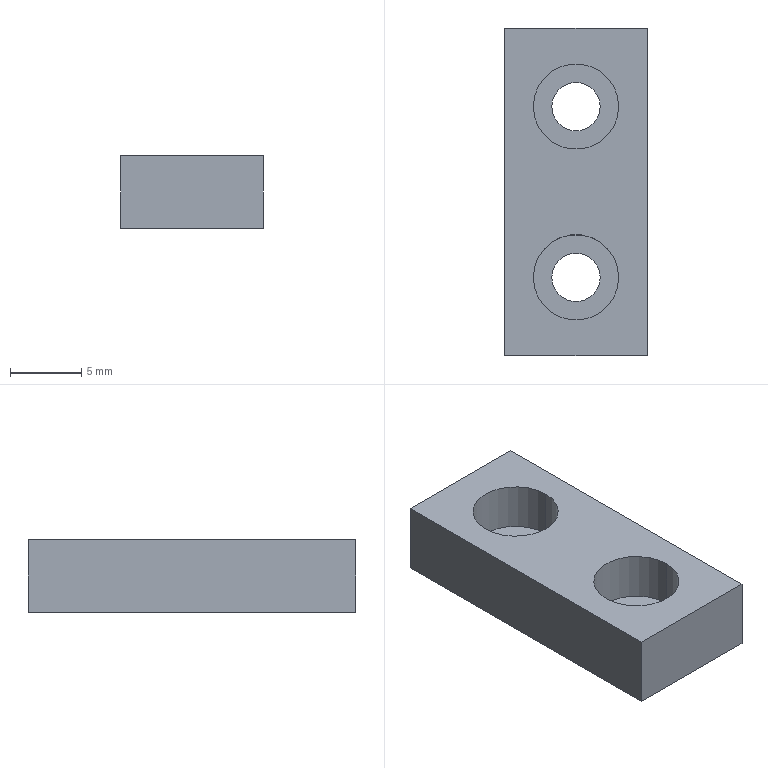Part | STEP file | 2041 Bag feed assist block | 1 solid | 16 faces | box 10 x 23 x 5.1 mm | volume 949.865 mm3 | cylinder 8 | plane 8 | commonest cylinder face diameters 3.4 x4 6 x4
STEP:
#1=CARTESIAN_POINT('',(0.,0.,0.));
#2=DIRECTION('',(0.,0.,1.));
#3=DIRECTION('',(1.,0.,0.));
#4=AXIS2_PLACEMENT_3D('',#1,#2,#3);
#5=CARTESIAN_POINT('',(3.,6.,1.7));
#6=VERTEX_POINT('',#5);
#7=CARTESIAN_POINT('',(3.,6.,5.1));
#8=VERTEX_POINT('',#7);
#9=CARTESIAN_POINT('',(3.,6.,5.1));
#10=DIRECTION('',(0.,0.,1.));
#11=VECTOR('',#10,1.);
#12=LINE('',#9,#11);
#13=CARTESIAN_POINT('',(0.,6.,5.1));
#14=DIRECTION('',(0.,0.,1.));
#15=DIRECTION('',(1.,0.,0.));
#16=AXIS2_PLACEMENT_3D('',#13,#14,#15);
#17=CYLINDRICAL_SURFACE('',#16,3.);
#18=CARTESIAN_POINT('',(6.283,0.));
#19=DIRECTION('',(0.,1.));
#20=VECTOR('',#19,1.);
#21=LINE('',#18,#20);
#22=(GEOMETRIC_REPRESENTATION_CONTEXT(2)PARAMETRIC_REPRESENTATION_CONTEXT()REPRESENTATION_CONTEXT('',''));
#23=DEFINITIONAL_REPRESENTATION('',(#21),#22);
#24=PCURVE('',#17,#23);
#25=CARTESIAN_POINT('',(0.,6.,5.1));
#26=DIRECTION('',(0.,0.,1.));
#27=DIRECTION('',(1.,0.,0.));
#28=AXIS2_PLACEMENT_3D('',#25,#26,#27);
#29=CYLINDRICAL_SURFACE('',#28,3.);
#30=CARTESIAN_POINT('',(0.,0.));
#31=DIRECTION('',(0.,1.));
#32=VECTOR('',#31,1.);
#33=LINE('',#30,#32);
#34=(GEOMETRIC_REPRESENTATION_CONTEXT(2)PARAMETRIC_REPRESENTATION_CONTEXT()REPRESENTATION_CONTEXT('',''));
#35=DEFINITIONAL_REPRESENTATION('',(#33),#34);
#36=PCURVE('',#29,#35);
#37=SURFACE_CURVE('',#12,(#24,#36),.PCURVE_S1.);
#38=EDGE_CURVE('',#6,#8,#37,.T.);
#39=ORIENTED_EDGE('',*,*,#38,.T.);
#40=CARTESIAN_POINT('',(-3.,6.,5.1));
#41=VERTEX_POINT('',#40);
#42=CARTESIAN_POINT('',(0.,6.,5.1));
#43=DIRECTION('',(0.,0.,1.));
#44=DIRECTION('',(1.,0.,0.));
#45=AXIS2_PLACEMENT_3D('',#42,#43,#44);
#46=CIRCLE('',#45,3.);
#47=CARTESIAN_POINT('',(0.,0.));
#48=DIRECTION('',(1.,0.));
#49=VECTOR('',#48,1.);
#50=LINE('',#47,#49);
#51=(GEOMETRIC_REPRESENTATION_CONTEXT(2)PARAMETRIC_REPRESENTATION_CONTEXT()REPRESENTATION_CONTEXT('',''));
#52=DEFINITIONAL_REPRESENTATION('',(#50),#51);
#53=PCURVE('',#17,#52);
#54=CARTESIAN_POINT('',(0.,0.,5.1));
#55=DIRECTION('',(0.,0.,-1.));
#56=DIRECTION('',(-1.,0.,0.));
#57=AXIS2_PLACEMENT_3D('',#54,#55,#56);
#58=PLANE('',#57);
#59=CARTESIAN_POINT('',(-3.,6.));
#60=CARTESIAN_POINT('',(-3.,11.196));
#61=CARTESIAN_POINT('',(1.5,8.598));
#62=CARTESIAN_POINT('',(6.,6.));
#63=CARTESIAN_POINT('',(1.5,3.402));
#64=CARTESIAN_POINT('',(-3.,0.8038));
#65=CARTESIAN_POINT('',(-3.,6.));
#66=(BOUNDED_CURVE()B_SPLINE_CURVE(2,(#59,#60,#61,#62,#63,#64,#65),.UNSPECIFIED.,.T.,.F.)B_SPLINE_CURVE_WITH_KNOTS((1,2,2,2,2,1),(-2.094,0.,2.094,4.189,6.283,8.378),.UNSPECIFIED.)CURVE()GEOMETRIC_REPRESENTATION_ITEM()RATIONAL_B_SPLINE_CURVE((1.,0.5,1.,0.5,1.,0.5,1.))REPRESENTATION_ITEM(''));
#67=(GEOMETRIC_REPRESENTATION_CONTEXT(2)PARAMETRIC_REPRESENTATION_CONTEXT()REPRESENTATION_CONTEXT('',''));
#68=DEFINITIONAL_REPRESENTATION('',(#66),#67);
#69=PCURVE('',#58,#68);
#70=SURFACE_CURVE('',#46,(#53,#69),.PCURVE_S1.);
#71=EDGE_CURVE('',#41,#8,#70,.T.);
#72=ORIENTED_EDGE('',*,*,#71,.F.);
#73=CARTESIAN_POINT('',(-3.,6.,1.7));
#74=VERTEX_POINT('',#73);
#75=CARTESIAN_POINT('',(-3.,6.,5.1));
#76=DIRECTION('',(0.,0.,1.));
#77=VECTOR('',#76,1.);
#78=LINE('',#75,#77);
#79=CARTESIAN_POINT('',(3.142,0.));
#80=DIRECTION('',(0.,1.));
#81=VECTOR('',#80,1.);
#82=LINE('',#79,#81);
#83=(GEOMETRIC_REPRESENTATION_CONTEXT(2)PARAMETRIC_REPRESENTATION_CONTEXT()REPRESENTATION_CONTEXT('',''));
#84=DEFINITIONAL_REPRESENTATION('',(#82),#83);
#85=PCURVE('',#17,#84);
#86=CARTESIAN_POINT('',(3.142,0.));
#87=DIRECTION('',(0.,1.));
#88=VECTOR('',#87,1.);
#89=LINE('',#86,#88);
#90=(GEOMETRIC_REPRESENTATION_CONTEXT(2)PARAMETRIC_REPRESENTATION_CONTEXT()REPRESENTATION_CONTEXT('',''));
#91=DEFINITIONAL_REPRESENTATION('',(#89),#90);
#92=PCURVE('',#29,#91);
#93=SURFACE_CURVE('',#78,(#85,#92),.PCURVE_S1.);
#94=EDGE_CURVE('',#74,#41,#93,.T.);
#95=ORIENTED_EDGE('',*,*,#94,.F.);
#96=CARTESIAN_POINT('',(0.,6.,1.7));
#97=DIRECTION('',(0.,0.,1.));
#98=DIRECTION('',(1.,0.,0.));
#99=AXIS2_PLACEMENT_3D('',#96,#97,#98);
#100=CIRCLE('',#99,3.);
#101=CARTESIAN_POINT('',(0.,-3.4));
#102=DIRECTION('',(1.,0.));
#103=VECTOR('',#102,1.);
#104=LINE('',#101,#103);
#105=(GEOMETRIC_REPRESENTATION_CONTEXT(2)PARAMETRIC_REPRESENTATION_CONTEXT()REPRESENTATION_CONTEXT('',''));
#106=DEFINITIONAL_REPRESENTATION('',(#104),#105);
#107=PCURVE('',#17,#106);
#108=CARTESIAN_POINT('',(1.7,6.,1.7));
#109=DIRECTION('',(0.,0.,-1.));
#110=DIRECTION('',(-1.,0.,0.));
#111=AXIS2_PLACEMENT_3D('',#108,#109,#110);
#112=PLANE('',#111);
#113=CARTESIAN_POINT('',(-1.3,0.));
#114=CARTESIAN_POINT('',(-1.3,5.196));
#115=CARTESIAN_POINT('',(3.2,2.598));
#116=CARTESIAN_POINT('',(7.7,0.));
#117=CARTESIAN_POINT('',(3.2,-2.598));
#118=CARTESIAN_POINT('',(-1.3,-5.196));
#119=CARTESIAN_POINT('',(-1.3,0.));
#120=(BOUNDED_CURVE()B_SPLINE_CURVE(2,(#113,#114,#115,#116,#117,#118,#119),.UNSPECIFIED.,.T.,.F.)B_SPLINE_CURVE_WITH_KNOTS((1,2,2,2,2,1),(-2.094,0.,2.094,4.189,6.283,8.378),.UNSPECIFIED.)CURVE()GEOMETRIC_REPRESENTATION_ITEM()RATIONAL_B_SPLINE_CURVE((1.,0.5,1.,0.5,1.,0.5,1.))REPRESENTATION_ITEM(''));
#121=(GEOMETRIC_REPRESENTATION_CONTEXT(2)PARAMETRIC_REPRESENTATION_CONTEXT()REPRESENTATION_CONTEXT('',''));
#122=DEFINITIONAL_REPRESENTATION('',(#120),#121);
#123=PCURVE('',#112,#122);
#124=SURFACE_CURVE('',#100,(#107,#123),.PCURVE_S1.);
#125=EDGE_CURVE('',#74,#6,#124,.T.);
#126=ORIENTED_EDGE('',*,*,#125,.T.);
#127=EDGE_LOOP('',(#39,#72,#95,#126));
#128=FACE_BOUND('',#127,.F.);
#129=ADVANCED_FACE('',(#128),#17,.F.);
#130=CARTESIAN_POINT('',(1.7,6.,0.));
#131=VERTEX_POINT('',#130);
#132=CARTESIAN_POINT('',(1.7,6.,1.7));
#133=VERTEX_POINT('',#132);
#134=CARTESIAN_POINT('',(1.7,6.,5.1));
#135=DIRECTION('',(0.,0.,1.));
#136=VECTOR('',#135,1.);
#137=LINE('',#134,#136);
#138=CARTESIAN_POINT('',(0.,6.,5.1));
#139=DIRECTION('',(0.,0.,1.));
#140=DIRECTION('',(1.,0.,0.));
#141=AXIS2_PLACEMENT_3D('',#138,#139,#140);
#142=CYLINDRICAL_SURFACE('',#141,1.7);
#143=CARTESIAN_POINT('',(6.283,0.));
#144=DIRECTION('',(0.,1.));
#145=VECTOR('',#144,1.);
#146=LINE('',#143,#145);
#147=(GEOMETRIC_REPRESENTATION_CONTEXT(2)PARAMETRIC_REPRESENTATION_CONTEXT()REPRESENTATION_CONTEXT('',''));
#148=DEFINITIONAL_REPRESENTATION('',(#146),#147);
#149=PCURVE('',#142,#148);
#150=CARTESIAN_POINT('',(0.,6.,5.1));
#151=DIRECTION('',(0.,0.,1.));
#152=DIRECTION('',(1.,0.,0.));
#153=AXIS2_PLACEMENT_3D('',#150,#151,#152);
#154=CYLINDRICAL_SURFACE('',#153,1.7);
#155=CARTESIAN_POINT('',(0.,0.));
#156=DIRECTION('',(0.,1.));
#157=VECTOR('',#156,1.);
#158=LINE('',#155,#157);
#159=(GEOMETRIC_REPRESENTATION_CONTEXT(2)PARAMETRIC_REPRESENTATION_CONTEXT()REPRESENTATION_CONTEXT('',''));
#160=DEFINITIONAL_REPRESENTATION('',(#158),#159);
#161=PCURVE('',#154,#160);
#162=SURFACE_CURVE('',#137,(#149,#161),.PCURVE_S1.);
#163=EDGE_CURVE('',#131,#133,#162,.T.);
#164=ORIENTED_EDGE('',*,*,#163,.T.);
#165=CARTESIAN_POINT('',(-1.7,6.,1.7));
#166=VERTEX_POINT('',#165);
#167=CARTESIAN_POINT('',(0.,6.,1.7));
#168=DIRECTION('',(0.,0.,1.));
#169=DIRECTION('',(1.,0.,0.));
#170=AXIS2_PLACEMENT_3D('',#167,#168,#169);
#171=CIRCLE('',#170,1.7);
#172=CARTESIAN_POINT('',(0.,-3.4));
#173=DIRECTION('',(1.,0.));
#174=VECTOR('',#173,1.);
#175=LINE('',#172,#174);
#176=(GEOMETRIC_REPRESENTATION_CONTEXT(2)PARAMETRIC_REPRESENTATION_CONTEXT()REPRESENTATION_CONTEXT('',''));
#177=DEFINITIONAL_REPRESENTATION('',(#175),#176);
#178=PCURVE('',#142,#177);
#179=CARTESIAN_POINT('',(0.,0.));
#180=CARTESIAN_POINT('',(0.,2.944));
#181=CARTESIAN_POINT('',(2.55,1.472));
#182=CARTESIAN_POINT('',(5.1,0.));
#183=CARTESIAN_POINT('',(2.55,-1.472));
#184=CARTESIAN_POINT('',(0.,-2.944));
#185=CARTESIAN_POINT('',(0.,0.));
#186=(BOUNDED_CURVE()B_SPLINE_CURVE(2,(#179,#180,#181,#182,#183,#184,#185),.UNSPECIFIED.,.T.,.F.)B_SPLINE_CURVE_WITH_KNOTS((1,2,2,2,2,1),(-2.094,0.,2.094,4.189,6.283,8.378),.UNSPECIFIED.)CURVE()GEOMETRIC_REPRESENTATION_ITEM()RATIONAL_B_SPLINE_CURVE((1.,0.5,1.,0.5,1.,0.5,1.))REPRESENTATION_ITEM(''));
#187=(GEOMETRIC_REPRESENTATION_CONTEXT(2)PARAMETRIC_REPRESENTATION_CONTEXT()REPRESENTATION_CONTEXT('',''));
#188=DEFINITIONAL_REPRESENTATION('',(#186),#187);
#189=PCURVE('',#112,#188);
#190=SURFACE_CURVE('',#171,(#178,#189),.PCURVE_S1.);
#191=EDGE_CURVE('',#166,#133,#190,.T.);
#192=ORIENTED_EDGE('',*,*,#191,.F.);
#193=CARTESIAN_POINT('',(-1.7,6.,0.));
#194=VERTEX_POINT('',#193);
#195=CARTESIAN_POINT('',(-1.7,6.,5.1));
#196=DIRECTION('',(0.,0.,1.));
#197=VECTOR('',#196,1.);
#198=LINE('',#195,#197);
#199=CARTESIAN_POINT('',(3.142,0.));
#200=DIRECTION('',(0.,1.));
#201=VECTOR('',#200,1.);
#202=LINE('',#199,#201);
#203=(GEOMETRIC_REPRESENTATION_CONTEXT(2)PARAMETRIC_REPRESENTATION_CONTEXT()REPRESENTATION_CONTEXT('',''));
#204=DEFINITIONAL_REPRESENTATION('',(#202),#203);
#205=PCURVE('',#142,#204);
#206=CARTESIAN_POINT('',(3.142,0.));
#207=DIRECTION('',(0.,1.));
#208=VECTOR('',#207,1.);
#209=LINE('',#206,#208);
#210=(GEOMETRIC_REPRESENTATION_CONTEXT(2)PARAMETRIC_REPRESENTATION_CONTEXT()REPRESENTATION_CONTEXT('',''));
#211=DEFINITIONAL_REPRESENTATION('',(#209),#210);
#212=PCURVE('',#154,#211);
#213=SURFACE_CURVE('',#198,(#205,#212),.PCURVE_S1.);
#214=EDGE_CURVE('',#194,#166,#213,.T.);
#215=ORIENTED_EDGE('',*,*,#214,.F.);
#216=CARTESIAN_POINT('',(0.,6.,0.));
#217=DIRECTION('',(0.,0.,1.));
#218=DIRECTION('',(1.,0.,0.));
#219=AXIS2_PLACEMENT_3D('',#216,#217,#218);
#220=CIRCLE('',#219,1.7);
#221=CARTESIAN_POINT('',(0.,-5.1));
#222=DIRECTION('',(1.,0.));
#223=VECTOR('',#222,1.);
#224=LINE('',#221,#223);
#225=(GEOMETRIC_REPRESENTATION_CONTEXT(2)PARAMETRIC_REPRESENTATION_CONTEXT()REPRESENTATION_CONTEXT('',''));
#226=DEFINITIONAL_REPRESENTATION('',(#224),#225);
#227=PCURVE('',#142,#226);
#228=CARTESIAN_POINT('',(0.,0.,0.));
#229=DIRECTION('',(0.,0.,-1.));
#230=DIRECTION('',(-1.,0.,0.));
#231=AXIS2_PLACEMENT_3D('',#228,#229,#230);
#232=PLANE('',#231);
#233=CARTESIAN_POINT('',(-1.7,6.));
#234=CARTESIAN_POINT('',(-1.7,8.944));
#235=CARTESIAN_POINT('',(0.85,7.472));
#236=CARTESIAN_POINT('',(3.4,6.));
#237=CARTESIAN_POINT('',(0.85,4.528));
#238=CARTESIAN_POINT('',(-1.7,3.056));
#239=CARTESIAN_POINT('',(-1.7,6.));
#240=(BOUNDED_CURVE()B_SPLINE_CURVE(2,(#233,#234,#235,#236,#237,#238,#239),.UNSPECIFIED.,.T.,.F.)B_SPLINE_CURVE_WITH_KNOTS((1,2,2,2,2,1),(-2.094,0.,2.094,4.189,6.283,8.378),.UNSPECIFIED.)CURVE()GEOMETRIC_REPRESENTATION_ITEM()RATIONAL_B_SPLINE_CURVE((1.,0.5,1.,0.5,1.,0.5,1.))REPRESENTATION_ITEM(''));
#241=(GEOMETRIC_REPRESENTATION_CONTEXT(2)PARAMETRIC_REPRESENTATION_CONTEXT()REPRESENTATION_CONTEXT('',''));
#242=DEFINITIONAL_REPRESENTATION('',(#240),#241);
#243=PCURVE('',#232,#242);
#244=SURFACE_CURVE('',#220,(#227,#243),.PCURVE_S1.);
#245=EDGE_CURVE('',#194,#131,#244,.T.);
#246=ORIENTED_EDGE('',*,*,#245,.T.);
#247=EDGE_LOOP('',(#164,#192,#215,#246));
#248=FACE_BOUND('',#247,.F.);
#249=ADVANCED_FACE('',(#248),#142,.F.);
#250=CARTESIAN_POINT('',(3.,-6.,1.7));
#251=VERTEX_POINT('',#250);
#252=CARTESIAN_POINT('',(3.,-6.,5.1));
#253=VERTEX_POINT('',#252);
#254=CARTESIAN_POINT('',(3.,-6.,5.1));
#255=DIRECTION('',(0.,0.,1.));
#256=VECTOR('',#255,1.);
#257=LINE('',#254,#256);
#258=CARTESIAN_POINT('',(0.,-6.,5.1));
#259=DIRECTION('',(0.,0.,1.));
#260=DIRECTION('',(1.,0.,0.));
#261=AXIS2_PLACEMENT_3D('',#258,#259,#260);
#262=CYLINDRICAL_SURFACE('',#261,3.);
#263=CARTESIAN_POINT('',(6.283,0.));
#264=DIRECTION('',(0.,1.));
#265=VECTOR('',#264,1.);
#266=LINE('',#263,#265);
#267=(GEOMETRIC_REPRESENTATION_CONTEXT(2)PARAMETRIC_REPRESENTATION_CONTEXT()REPRESENTATION_CONTEXT('',''));
#268=DEFINITIONAL_REPRESENTATION('',(#266),#267);
#269=PCURVE('',#262,#268);
#270=CARTESIAN_POINT('',(0.,-6.,5.1));
#271=DIRECTION('',(0.,0.,1.));
#272=DIRECTION('',(1.,0.,0.));
#273=AXIS2_PLACEMENT_3D('',#270,#271,#272);
#274=CYLINDRICAL_SURFACE('',#273,3.);
#275=CARTESIAN_POINT('',(0.,0.));
#276=DIRECTION('',(0.,1.));
#277=VECTOR('',#276,1.);
#278=LINE('',#275,#277);
#279=(GEOMETRIC_REPRESENTATION_CONTEXT(2)PARAMETRIC_REPRESENTATION_CONTEXT()REPRESENTATION_CONTEXT('',''));
#280=DEFINITIONAL_REPRESENTATION('',(#278),#279);
#281=PCURVE('',#274,#280);
#282=SURFACE_CURVE('',#257,(#269,#281),.PCURVE_S1.);
#283=EDGE_CURVE('',#251,#253,#282,.T.);
#284=ORIENTED_EDGE('',*,*,#283,.T.);
#285=CARTESIAN_POINT('',(-3.,-6.,5.1));
#286=VERTEX_POINT('',#285);
#287=CARTESIAN_POINT('',(0.,-6.,5.1));
#288=DIRECTION('',(0.,0.,1.));
#289=DIRECTION('',(1.,0.,0.));
#290=AXIS2_PLACEMENT_3D('',#287,#288,#289);
#291=CIRCLE('',#290,3.);
#292=CARTESIAN_POINT('',(0.,0.));
#293=DIRECTION('',(1.,0.));
#294=VECTOR('',#293,1.);
#295=LINE('',#292,#294);
#296=(GEOMETRIC_REPRESENTATION_CONTEXT(2)PARAMETRIC_REPRESENTATION_CONTEXT()REPRESENTATION_CONTEXT('',''));
#297=DEFINITIONAL_REPRESENTATION('',(#295),#296);
#298=PCURVE('',#262,#297);
#299=CARTESIAN_POINT('',(-3.,-6.));
#300=CARTESIAN_POINT('',(-3.,-0.8038));
#301=CARTESIAN_POINT('',(1.5,-3.402));
#302=CARTESIAN_POINT('',(6.,-6.));
#303=CARTESIAN_POINT('',(1.5,-8.598));
#304=CARTESIAN_POINT('',(-3.,-11.196));
#305=CARTESIAN_POINT('',(-3.,-6.));
#306=(BOUNDED_CURVE()B_SPLINE_CURVE(2,(#299,#300,#301,#302,#303,#304,#305),.UNSPECIFIED.,.T.,.F.)B_SPLINE_CURVE_WITH_KNOTS((1,2,2,2,2,1),(-2.094,0.,2.094,4.189,6.283,8.378),.UNSPECIFIED.)CURVE()GEOMETRIC_REPRESENTATION_ITEM()RATIONAL_B_SPLINE_CURVE((1.,0.5,1.,0.5,1.,0.5,1.))REPRESENTATION_ITEM(''));
#307=(GEOMETRIC_REPRESENTATION_CONTEXT(2)PARAMETRIC_REPRESENTATION_CONTEXT()REPRESENTATION_CONTEXT('',''));
#308=DEFINITIONAL_REPRESENTATION('',(#306),#307);
#309=PCURVE('',#58,#308);
#310=SURFACE_CURVE('',#291,(#298,#309),.PCURVE_S1.);
#311=EDGE_CURVE('',#286,#253,#310,.T.);
#312=ORIENTED_EDGE('',*,*,#311,.F.);
#313=CARTESIAN_POINT('',(-3.,-6.,1.7));
#314=VERTEX_POINT('',#313);
#315=CARTESIAN_POINT('',(-3.,-6.,5.1));
#316=DIRECTION('',(0.,0.,1.));
#317=VECTOR('',#316,1.);
#318=LINE('',#315,#317);
#319=CARTESIAN_POINT('',(3.142,0.));
#320=DIRECTION('',(0.,1.));
#321=VECTOR('',#320,1.);
#322=LINE('',#319,#321);
#323=(GEOMETRIC_REPRESENTATION_CONTEXT(2)PARAMETRIC_REPRESENTATION_CONTEXT()REPRESENTATION_CONTEXT('',''));
#324=DEFINITIONAL_REPRESENTATION('',(#322),#323);
#325=PCURVE('',#262,#324);
#326=CARTESIAN_POINT('',(3.142,0.));
#327=DIRECTION('',(0.,1.));
#328=VECTOR('',#327,1.);
#329=LINE('',#326,#328);
#330=(GEOMETRIC_REPRESENTATION_CONTEXT(2)PARAMETRIC_REPRESENTATION_CONTEXT()REPRESENTATION_CONTEXT('',''));
#331=DEFINITIONAL_REPRESENTATION('',(#329),#330);
#332=PCURVE('',#274,#331);
#333=SURFACE_CURVE('',#318,(#325,#332),.PCURVE_S1.);
#334=EDGE_CURVE('',#314,#286,#333,.T.);
#335=ORIENTED_EDGE('',*,*,#334,.F.);
#336=CARTESIAN_POINT('',(0.,-6.,1.7));
#337=DIRECTION('',(0.,0.,1.));
#338=DIRECTION('',(1.,0.,0.));
#339=AXIS2_PLACEMENT_3D('',#336,#337,#338);
#340=CIRCLE('',#339,3.);
#341=CARTESIAN_POINT('',(0.,-3.4));
#342=DIRECTION('',(1.,0.));
#343=VECTOR('',#342,1.);
#344=LINE('',#341,#343);
#345=(GEOMETRIC_REPRESENTATION_CONTEXT(2)PARAMETRIC_REPRESENTATION_CONTEXT()REPRESENTATION_CONTEXT('',''));
#346=DEFINITIONAL_REPRESENTATION('',(#344),#345);
#347=PCURVE('',#262,#346);
#348=CARTESIAN_POINT('',(1.7,-6.,1.7));
#349=DIRECTION('',(0.,0.,-1.));
#350=DIRECTION('',(-1.,0.,0.));
#351=AXIS2_PLACEMENT_3D('',#348,#349,#350);
#352=PLANE('',#351);
#353=CARTESIAN_POINT('',(-1.3,0.));
#354=CARTESIAN_POINT('',(-1.3,5.196));
#355=CARTESIAN_POINT('',(3.2,2.598));
#356=CARTESIAN_POINT('',(7.7,0.));
#357=CARTESIAN_POINT('',(3.2,-2.598));
#358=CARTESIAN_POINT('',(-1.3,-5.196));
#359=CARTESIAN_POINT('',(-1.3,0.));
#360=(BOUNDED_CURVE()B_SPLINE_CURVE(2,(#353,#354,#355,#356,#357,#358,#359),.UNSPECIFIED.,.T.,.F.)B_SPLINE_CURVE_WITH_KNOTS((1,2,2,2,2,1),(-2.094,0.,2.094,4.189,6.283,8.378),.UNSPECIFIED.)CURVE()GEOMETRIC_REPRESENTATION_ITEM()RATIONAL_B_SPLINE_CURVE((1.,0.5,1.,0.5,1.,0.5,1.))REPRESENTATION_ITEM(''));
#361=(GEOMETRIC_REPRESENTATION_CONTEXT(2)PARAMETRIC_REPRESENTATION_CONTEXT()REPRESENTATION_CONTEXT('',''));
#362=DEFINITIONAL_REPRESENTATION('',(#360),#361);
#363=PCURVE('',#352,#362);
#364=SURFACE_CURVE('',#340,(#347,#363),.PCURVE_S1.);
#365=EDGE_CURVE('',#314,#251,#364,.T.);
#366=ORIENTED_EDGE('',*,*,#365,.T.);
#367=EDGE_LOOP('',(#284,#312,#335,#366));
#368=FACE_BOUND('',#367,.F.);
#369=ADVANCED_FACE('',(#368),#262,.F.);
#370=CARTESIAN_POINT('',(1.7,-6.,0.));
#371=VERTEX_POINT('',#370);
#372=CARTESIAN_POINT('',(1.7,-6.,1.7));
#373=VERTEX_POINT('',#372);
#374=CARTESIAN_POINT('',(1.7,-6.,5.1));
#375=DIRECTION('',(0.,0.,1.));
#376=VECTOR('',#375,1.);
#377=LINE('',#374,#376);
#378=CARTESIAN_POINT('',(0.,-6.,5.1));
#379=DIRECTION('',(0.,0.,1.));
#380=DIRECTION('',(1.,0.,0.));
#381=AXIS2_PLACEMENT_3D('',#378,#379,#380);
#382=CYLINDRICAL_SURFACE('',#381,1.7);
#383=CARTESIAN_POINT('',(6.283,0.));
#384=DIRECTION('',(0.,1.));
#385=VECTOR('',#384,1.);
#386=LINE('',#383,#385);
#387=(GEOMETRIC_REPRESENTATION_CONTEXT(2)PARAMETRIC_REPRESENTATION_CONTEXT()REPRESENTATION_CONTEXT('',''));
#388=DEFINITIONAL_REPRESENTATION('',(#386),#387);
#389=PCURVE('',#382,#388);
#390=CARTESIAN_POINT('',(0.,-6.,5.1));
#391=DIRECTION('',(0.,0.,1.));
#392=DIRECTION('',(1.,0.,0.));
#393=AXIS2_PLACEMENT_3D('',#390,#391,#392);
#394=CYLINDRICAL_SURFACE('',#393,1.7);
#395=CARTESIAN_POINT('',(0.,0.));
#396=DIRECTION('',(0.,1.));
#397=VECTOR('',#396,1.);
#398=LINE('',#395,#397);
#399=(GEOMETRIC_REPRESENTATION_CONTEXT(2)PARAMETRIC_REPRESENTATION_CONTEXT()REPRESENTATION_CONTEXT('',''));
#400=DEFINITIONAL_REPRESENTATION('',(#398),#399);
#401=PCURVE('',#394,#400);
#402=SURFACE_CURVE('',#377,(#389,#401),.PCURVE_S1.);
#403=EDGE_CURVE('',#371,#373,#402,.T.);
#404=ORIENTED_EDGE('',*,*,#403,.T.);
#405=CARTESIAN_POINT('',(-1.7,-6.,1.7));
#406=VERTEX_POINT('',#405);
#407=CARTESIAN_POINT('',(0.,-6.,1.7));
#408=DIRECTION('',(0.,0.,1.));
#409=DIRECTION('',(1.,0.,0.));
#410=AXIS2_PLACEMENT_3D('',#407,#408,#409);
#411=CIRCLE('',#410,1.7);
#412=CARTESIAN_POINT('',(0.,-3.4));
#413=DIRECTION('',(1.,0.));
#414=VECTOR('',#413,1.);
#415=LINE('',#412,#414);
#416=(GEOMETRIC_REPRESENTATION_CONTEXT(2)PARAMETRIC_REPRESENTATION_CONTEXT()REPRESENTATION_CONTEXT('',''));
#417=DEFINITIONAL_REPRESENTATION('',(#415),#416);
#418=PCURVE('',#382,#417);
#419=CARTESIAN_POINT('',(0.,0.));
#420=CARTESIAN_POINT('',(0.,2.944));
#421=CARTESIAN_POINT('',(2.55,1.472));
#422=CARTESIAN_POINT('',(5.1,0.));
#423=CARTESIAN_POINT('',(2.55,-1.472));
#424=CARTESIAN_POINT('',(0.,-2.944));
#425=CARTESIAN_POINT('',(0.,0.));
#426=(BOUNDED_CURVE()B_SPLINE_CURVE(2,(#419,#420,#421,#422,#423,#424,#425),.UNSPECIFIED.,.T.,.F.)B_SPLINE_CURVE_WITH_KNOTS((1,2,2,2,2,1),(-2.094,0.,2.094,4.189,6.283,8.378),.UNSPECIFIED.)CURVE()GEOMETRIC_REPRESENTATION_ITEM()RATIONAL_B_SPLINE_CURVE((1.,0.5,1.,0.5,1.,0.5,1.))REPRESENTATION_ITEM(''));
#427=(GEOMETRIC_REPRESENTATION_CONTEXT(2)PARAMETRIC_REPRESENTATION_CONTEXT()REPRESENTATION_CONTEXT('',''));
#428=DEFINITIONAL_REPRESENTATION('',(#426),#427);
#429=PCURVE('',#352,#428);
#430=SURFACE_CURVE('',#411,(#418,#429),.PCURVE_S1.);
#431=EDGE_CURVE('',#406,#373,#430,.T.);
#432=ORIENTED_EDGE('',*,*,#431,.F.);
#433=CARTESIAN_POINT('',(-1.7,-6.,0.));
#434=VERTEX_POINT('',#433);
#435=CARTESIAN_POINT('',(-1.7,-6.,5.1));
#436=DIRECTION('',(0.,0.,1.));
#437=VECTOR('',#436,1.);
#438=LINE('',#435,#437);
#439=CARTESIAN_POINT('',(3.142,0.));
#440=DIRECTION('',(0.,1.));
#441=VECTOR('',#440,1.);
#442=LINE('',#439,#441);
#443=(GEOMETRIC_REPRESENTATION_CONTEXT(2)PARAMETRIC_REPRESENTATION_CONTEXT()REPRESENTATION_CONTEXT('',''));
#444=DEFINITIONAL_REPRESENTATION('',(#442),#443);
#445=PCURVE('',#382,#444);
#446=CARTESIAN_POINT('',(3.142,0.));
#447=DIRECTION('',(0.,1.));
#448=VECTOR('',#447,1.);
#449=LINE('',#446,#448);
#450=(GEOMETRIC_REPRESENTATION_CONTEXT(2)PARAMETRIC_REPRESENTATION_CONTEXT()REPRESENTATION_CONTEXT('',''));
#451=DEFINITIONAL_REPRESENTATION('',(#449),#450);
#452=PCURVE('',#394,#451);
#453=SURFACE_CURVE('',#438,(#445,#452),.PCURVE_S1.);
#454=EDGE_CURVE('',#434,#406,#453,.T.);
#455=ORIENTED_EDGE('',*,*,#454,.F.);
#456=CARTESIAN_POINT('',(0.,-6.,0.));
#457=DIRECTION('',(0.,0.,1.));
#458=DIRECTION('',(1.,0.,0.));
#459=AXIS2_PLACEMENT_3D('',#456,#457,#458);
#460=CIRCLE('',#459,1.7);
#461=CARTESIAN_POINT('',(0.,-5.1));
#462=DIRECTION('',(1.,0.));
#463=VECTOR('',#462,1.);
#464=LINE('',#461,#463);
#465=(GEOMETRIC_REPRESENTATION_CONTEXT(2)PARAMETRIC_REPRESENTATION_CONTEXT()REPRESENTATION_CONTEXT('',''));
#466=DEFINITIONAL_REPRESENTATION('',(#464),#465);
#467=PCURVE('',#382,#466);
#468=CARTESIAN_POINT('',(-1.7,-6.));
#469=CARTESIAN_POINT('',(-1.7,-3.056));
#470=CARTESIAN_POINT('',(0.85,-4.528));
#471=CARTESIAN_POINT('',(3.4,-6.));
#472=CARTESIAN_POINT('',(0.85,-7.472));
#473=CARTESIAN_POINT('',(-1.7,-8.944));
#474=CARTESIAN_POINT('',(-1.7,-6.));
#475=(BOUNDED_CURVE()B_SPLINE_CURVE(2,(#468,#469,#470,#471,#472,#473,#474),.UNSPECIFIED.,.T.,.F.)B_SPLINE_CURVE_WITH_KNOTS((1,2,2,2,2,1),(-2.094,0.,2.094,4.189,6.283,8.378),.UNSPECIFIED.)CURVE()GEOMETRIC_REPRESENTATION_ITEM()RATIONAL_B_SPLINE_CURVE((1.,0.5,1.,0.5,1.,0.5,1.))REPRESENTATION_ITEM(''));
#476=(GEOMETRIC_REPRESENTATION_CONTEXT(2)PARAMETRIC_REPRESENTATION_CONTEXT()REPRESENTATION_CONTEXT('',''));
#477=DEFINITIONAL_REPRESENTATION('',(#475),#476);
#478=PCURVE('',#232,#477);
#479=SURFACE_CURVE('',#460,(#467,#478),.PCURVE_S1.);
#480=EDGE_CURVE('',#434,#371,#479,.T.);
#481=ORIENTED_EDGE('',*,*,#480,.T.);
#482=EDGE_LOOP('',(#404,#432,#455,#481));
#483=FACE_BOUND('',#482,.F.);
#484=ADVANCED_FACE('',(#483),#382,.F.);
#485=CARTESIAN_POINT('',(5.,-11.5,0.));
#486=VERTEX_POINT('',#485);
#487=CARTESIAN_POINT('',(5.,11.5,0.));
#488=VERTEX_POINT('',#487);
#489=CARTESIAN_POINT('',(5.,-11.5,0.));
#490=DIRECTION('',(0.,1.,0.));
#491=VECTOR('',#490,1.);
#492=LINE('',#489,#491);
#493=CARTESIAN_POINT('',(5.,-11.5,5.1));
#494=DIRECTION('',(-1.,0.,0.));
#495=DIRECTION('',(0.,0.,1.));
#496=AXIS2_PLACEMENT_3D('',#493,#494,#495);
#497=PLANE('',#496);
#498=CARTESIAN_POINT('',(-5.1,0.));
#499=DIRECTION('',(0.,1.));
#500=VECTOR('',#499,1.);
#501=LINE('',#498,#500);
#502=(GEOMETRIC_REPRESENTATION_CONTEXT(2)PARAMETRIC_REPRESENTATION_CONTEXT()REPRESENTATION_CONTEXT('',''));
#503=DEFINITIONAL_REPRESENTATION('',(#501),#502);
#504=PCURVE('',#497,#503);
#505=CARTESIAN_POINT('',(-5.,-11.5));
#506=DIRECTION('',(0.,1.));
#507=VECTOR('',#506,1.);
#508=LINE('',#505,#507);
#509=(GEOMETRIC_REPRESENTATION_CONTEXT(2)PARAMETRIC_REPRESENTATION_CONTEXT()REPRESENTATION_CONTEXT('',''));
#510=DEFINITIONAL_REPRESENTATION('',(#508),#509);
#511=PCURVE('',#232,#510);
#512=SURFACE_CURVE('',#492,(#504,#511),.PCURVE_S1.);
#513=EDGE_CURVE('',#486,#488,#512,.T.);
#514=ORIENTED_EDGE('',*,*,#513,.T.);
#515=CARTESIAN_POINT('',(5.,11.5,5.1));
#516=VERTEX_POINT('',#515);
#517=CARTESIAN_POINT('',(5.,11.5,5.1));
#518=DIRECTION('',(0.,0.,-1.));
#519=VECTOR('',#518,1.);
#520=LINE('',#517,#519);
#521=CARTESIAN_POINT('',(0.,23.));
#522=DIRECTION('',(-1.,0.));
#523=VECTOR('',#522,1.);
#524=LINE('',#521,#523);
#525=(GEOMETRIC_REPRESENTATION_CONTEXT(2)PARAMETRIC_REPRESENTATION_CONTEXT()REPRESENTATION_CONTEXT('',''));
#526=DEFINITIONAL_REPRESENTATION('',(#524),#525);
#527=PCURVE('',#497,#526);
#528=CARTESIAN_POINT('',(-5.,11.5,5.1));
#529=DIRECTION('',(0.,-1.,0.));
#530=DIRECTION('',(0.,0.,-1.));
#531=AXIS2_PLACEMENT_3D('',#528,#529,#530);
#532=PLANE('',#531);
#533=CARTESIAN_POINT('',(0.,10.));
#534=DIRECTION('',(1.,0.));
#535=VECTOR('',#534,1.);
#536=LINE('',#533,#535);
#537=(GEOMETRIC_REPRESENTATION_CONTEXT(2)PARAMETRIC_REPRESENTATION_CONTEXT()REPRESENTATION_CONTEXT('',''));
#538=DEFINITIONAL_REPRESENTATION('',(#536),#537);
#539=PCURVE('',#532,#538);
#540=SURFACE_CURVE('',#520,(#527,#539),.PCURVE_S1.);
#541=EDGE_CURVE('',#516,#488,#540,.T.);
#542=ORIENTED_EDGE('',*,*,#541,.F.);
#543=CARTESIAN_POINT('',(5.,-11.5,5.1));
#544=VERTEX_POINT('',#543);
#545=CARTESIAN_POINT('',(5.,-11.5,5.1));
#546=DIRECTION('',(0.,1.,0.));
#547=VECTOR('',#546,1.);
#548=LINE('',#545,#547);
#549=CARTESIAN_POINT('',(0.,0.));
#550=DIRECTION('',(0.,1.));
#551=VECTOR('',#550,1.);
#552=LINE('',#549,#551);
#553=(GEOMETRIC_REPRESENTATION_CONTEXT(2)PARAMETRIC_REPRESENTATION_CONTEXT()REPRESENTATION_CONTEXT('',''));
#554=DEFINITIONAL_REPRESENTATION('',(#552),#553);
#555=PCURVE('',#497,#554);
#556=CARTESIAN_POINT('',(-5.,-11.5));
#557=DIRECTION('',(0.,1.));
#558=VECTOR('',#557,1.);
#559=LINE('',#556,#558);
#560=(GEOMETRIC_REPRESENTATION_CONTEXT(2)PARAMETRIC_REPRESENTATION_CONTEXT()REPRESENTATION_CONTEXT('',''));
#561=DEFINITIONAL_REPRESENTATION('',(#559),#560);
#562=PCURVE('',#58,#561);
#563=SURFACE_CURVE('',#548,(#555,#562),.PCURVE_S1.);
#564=EDGE_CURVE('',#544,#516,#563,.T.);
#565=ORIENTED_EDGE('',*,*,#564,.F.);
#566=CARTESIAN_POINT('',(5.,-11.5,5.1));
#567=DIRECTION('',(0.,0.,-1.));
#568=VECTOR('',#567,1.);
#569=LINE('',#566,#568);
#570=CARTESIAN_POINT('',(0.,0.));
#571=DIRECTION('',(-1.,0.));
#572=VECTOR('',#571,1.);
#573=LINE('',#570,#572);
#574=(GEOMETRIC_REPRESENTATION_CONTEXT(2)PARAMETRIC_REPRESENTATION_CONTEXT()REPRESENTATION_CONTEXT('',''));
#575=DEFINITIONAL_REPRESENTATION('',(#573),#574);
#576=PCURVE('',#497,#575);
#577=CARTESIAN_POINT('',(-5.,-11.5,5.1));
#578=DIRECTION('',(0.,1.,0.));
#579=DIRECTION('',(0.,0.,1.));
#580=AXIS2_PLACEMENT_3D('',#577,#578,#579);
#581=PLANE('',#580);
#582=CARTESIAN_POINT('',(0.,10.));
#583=DIRECTION('',(-1.,0.));
#584=VECTOR('',#583,1.);
#585=LINE('',#582,#584);
#586=(GEOMETRIC_REPRESENTATION_CONTEXT(2)PARAMETRIC_REPRESENTATION_CONTEXT()REPRESENTATION_CONTEXT('',''));
#587=DEFINITIONAL_REPRESENTATION('',(#585),#586);
#588=PCURVE('',#581,#587);
#589=SURFACE_CURVE('',#569,(#576,#588),.PCURVE_S1.);
#590=EDGE_CURVE('',#544,#486,#589,.T.);
#591=ORIENTED_EDGE('',*,*,#590,.T.);
#592=EDGE_LOOP('',(#514,#542,#565,#591));
#593=FACE_BOUND('',#592,.T.);
#594=ADVANCED_FACE('',(#593),#497,.F.);
#595=CARTESIAN_POINT('',(-5.,11.5,0.));
#596=VERTEX_POINT('',#595);
#597=CARTESIAN_POINT('',(-5.,11.5,0.));
#598=DIRECTION('',(-1.,0.,0.));
#599=VECTOR('',#598,1.);
#600=LINE('',#597,#599);
#601=CARTESIAN_POINT('',(5.1,0.));
#602=DIRECTION('',(0.,-1.));
#603=VECTOR('',#602,1.);
#604=LINE('',#601,#603);
#605=(GEOMETRIC_REPRESENTATION_CONTEXT(2)PARAMETRIC_REPRESENTATION_CONTEXT()REPRESENTATION_CONTEXT('',''));
#606=DEFINITIONAL_REPRESENTATION('',(#604),#605);
#607=PCURVE('',#532,#606);
#608=CARTESIAN_POINT('',(5.,11.5));
#609=DIRECTION('',(1.,0.));
#610=VECTOR('',#609,1.);
#611=LINE('',#608,#610);
#612=(GEOMETRIC_REPRESENTATION_CONTEXT(2)PARAMETRIC_REPRESENTATION_CONTEXT()REPRESENTATION_CONTEXT('',''));
#613=DEFINITIONAL_REPRESENTATION('',(#611),#612);
#614=PCURVE('',#232,#613);
#615=SURFACE_CURVE('',#600,(#607,#614),.PCURVE_S1.);
#616=EDGE_CURVE('',#488,#596,#615,.T.);
#617=ORIENTED_EDGE('',*,*,#616,.T.);
#618=CARTESIAN_POINT('',(-5.,11.5,5.1));
#619=VERTEX_POINT('',#618);
#620=CARTESIAN_POINT('',(-5.,11.5,5.1));
#621=DIRECTION('',(0.,0.,-1.));
#622=VECTOR('',#621,1.);
#623=LINE('',#620,#622);
#624=CARTESIAN_POINT('',(0.,0.));
#625=DIRECTION('',(1.,0.));
#626=VECTOR('',#625,1.);
#627=LINE('',#624,#626);
#628=(GEOMETRIC_REPRESENTATION_CONTEXT(2)PARAMETRIC_REPRESENTATION_CONTEXT()REPRESENTATION_CONTEXT('',''));
#629=DEFINITIONAL_REPRESENTATION('',(#627),#628);
#630=PCURVE('',#532,#629);
#631=CARTESIAN_POINT('',(-5.,-11.5,5.1));
#632=DIRECTION('',(1.,0.,0.));
#633=DIRECTION('',(0.,0.,-1.));
#634=AXIS2_PLACEMENT_3D('',#631,#632,#633);
#635=PLANE('',#634);
#636=CARTESIAN_POINT('',(0.,23.));
#637=DIRECTION('',(1.,0.));
#638=VECTOR('',#637,1.);
#639=LINE('',#636,#638);
#640=(GEOMETRIC_REPRESENTATION_CONTEXT(2)PARAMETRIC_REPRESENTATION_CONTEXT()REPRESENTATION_CONTEXT('',''));
#641=DEFINITIONAL_REPRESENTATION('',(#639),#640);
#642=PCURVE('',#635,#641);
#643=SURFACE_CURVE('',#623,(#630,#642),.PCURVE_S1.);
#644=EDGE_CURVE('',#619,#596,#643,.T.);
#645=ORIENTED_EDGE('',*,*,#644,.F.);
#646=CARTESIAN_POINT('',(-5.,11.5,5.1));
#647=DIRECTION('',(-1.,0.,0.));
#648=VECTOR('',#647,1.);
#649=LINE('',#646,#648);
#650=CARTESIAN_POINT('',(0.,0.));
#651=DIRECTION('',(0.,-1.));
#652=VECTOR('',#651,1.);
#653=LINE('',#650,#652);
#654=(GEOMETRIC_REPRESENTATION_CONTEXT(2)PARAMETRIC_REPRESENTATION_CONTEXT()REPRESENTATION_CONTEXT('',''));
#655=DEFINITIONAL_REPRESENTATION('',(#653),#654);
#656=PCURVE('',#532,#655);
#657=CARTESIAN_POINT('',(5.,11.5));
#658=DIRECTION('',(1.,0.));
#659=VECTOR('',#658,1.);
#660=LINE('',#657,#659);
#661=(GEOMETRIC_REPRESENTATION_CONTEXT(2)PARAMETRIC_REPRESENTATION_CONTEXT()REPRESENTATION_CONTEXT('',''));
#662=DEFINITIONAL_REPRESENTATION('',(#660),#661);
#663=PCURVE('',#58,#662);
#664=SURFACE_CURVE('',#649,(#656,#663),.PCURVE_S1.);
#665=EDGE_CURVE('',#516,#619,#664,.T.);
#666=ORIENTED_EDGE('',*,*,#665,.F.);
#667=ORIENTED_EDGE('',*,*,#541,.T.);
#668=EDGE_LOOP('',(#617,#645,#666,#667));
#669=FACE_BOUND('',#668,.T.);
#670=ADVANCED_FACE('',(#669),#532,.F.);
#671=CARTESIAN_POINT('',(-5.,-11.5,0.));
#672=VERTEX_POINT('',#671);
#673=CARTESIAN_POINT('',(-5.,-11.5,0.));
#674=DIRECTION('',(0.,-1.,0.));
#675=VECTOR('',#674,1.);
#676=LINE('',#673,#675);
#677=CARTESIAN_POINT('',(5.1,0.));
#678=DIRECTION('',(0.,-1.));
#679=VECTOR('',#678,1.);
#680=LINE('',#677,#679);
#681=(GEOMETRIC_REPRESENTATION_CONTEXT(2)PARAMETRIC_REPRESENTATION_CONTEXT()REPRESENTATION_CONTEXT('',''));
#682=DEFINITIONAL_REPRESENTATION('',(#680),#681);
#683=PCURVE('',#635,#682);
#684=CARTESIAN_POINT('',(5.,-11.5));
#685=DIRECTION('',(0.,-1.));
#686=VECTOR('',#685,1.);
#687=LINE('',#684,#686);
#688=(GEOMETRIC_REPRESENTATION_CONTEXT(2)PARAMETRIC_REPRESENTATION_CONTEXT()REPRESENTATION_CONTEXT('',''));
#689=DEFINITIONAL_REPRESENTATION('',(#687),#688);
#690=PCURVE('',#232,#689);
#691=SURFACE_CURVE('',#676,(#683,#690),.PCURVE_S1.);
#692=EDGE_CURVE('',#596,#672,#691,.T.);
#693=ORIENTED_EDGE('',*,*,#692,.T.);
#694=CARTESIAN_POINT('',(-5.,-11.5,5.1));
#695=VERTEX_POINT('',#694);
#696=CARTESIAN_POINT('',(-5.,-11.5,5.1));
#697=DIRECTION('',(0.,0.,-1.));
#698=VECTOR('',#697,1.);
#699=LINE('',#696,#698);
#700=CARTESIAN_POINT('',(0.,0.));
#701=DIRECTION('',(1.,0.));
#702=VECTOR('',#701,1.);
#703=LINE('',#700,#702);
#704=(GEOMETRIC_REPRESENTATION_CONTEXT(2)PARAMETRIC_REPRESENTATION_CONTEXT()REPRESENTATION_CONTEXT('',''));
#705=DEFINITIONAL_REPRESENTATION('',(#703),#704);
#706=PCURVE('',#635,#705);
#707=CARTESIAN_POINT('',(0.,0.));
#708=DIRECTION('',(-1.,0.));
#709=VECTOR('',#708,1.);
#710=LINE('',#707,#709);
#711=(GEOMETRIC_REPRESENTATION_CONTEXT(2)PARAMETRIC_REPRESENTATION_CONTEXT()REPRESENTATION_CONTEXT('',''));
#712=DEFINITIONAL_REPRESENTATION('',(#710),#711);
#713=PCURVE('',#581,#712);
#714=SURFACE_CURVE('',#699,(#706,#713),.PCURVE_S1.);
#715=EDGE_CURVE('',#695,#672,#714,.T.);
#716=ORIENTED_EDGE('',*,*,#715,.F.);
#717=CARTESIAN_POINT('',(-5.,-11.5,5.1));
#718=DIRECTION('',(0.,-1.,0.));
#719=VECTOR('',#718,1.);
#720=LINE('',#717,#719);
#721=CARTESIAN_POINT('',(0.,0.));
#722=DIRECTION('',(0.,-1.));
#723=VECTOR('',#722,1.);
#724=LINE('',#721,#723);
#725=(GEOMETRIC_REPRESENTATION_CONTEXT(2)PARAMETRIC_REPRESENTATION_CONTEXT()REPRESENTATION_CONTEXT('',''));
#726=DEFINITIONAL_REPRESENTATION('',(#724),#725);
#727=PCURVE('',#635,#726);
#728=CARTESIAN_POINT('',(5.,-11.5));
#729=DIRECTION('',(0.,-1.));
#730=VECTOR('',#729,1.);
#731=LINE('',#728,#730);
#732=(GEOMETRIC_REPRESENTATION_CONTEXT(2)PARAMETRIC_REPRESENTATION_CONTEXT()REPRESENTATION_CONTEXT('',''));
#733=DEFINITIONAL_REPRESENTATION('',(#731),#732);
#734=PCURVE('',#58,#733);
#735=SURFACE_CURVE('',#720,(#727,#734),.PCURVE_S1.);
#736=EDGE_CURVE('',#619,#695,#735,.T.);
#737=ORIENTED_EDGE('',*,*,#736,.F.);
#738=ORIENTED_EDGE('',*,*,#644,.T.);
#739=EDGE_LOOP('',(#693,#716,#737,#738));
#740=FACE_BOUND('',#739,.T.);
#741=ADVANCED_FACE('',(#740),#635,.F.);
#742=CARTESIAN_POINT('',(-5.,-11.5,0.));
#743=DIRECTION('',(1.,0.,0.));
#744=VECTOR('',#743,1.);
#745=LINE('',#742,#744);
#746=CARTESIAN_POINT('',(-5.1,0.));
#747=DIRECTION('',(0.,1.));
#748=VECTOR('',#747,1.);
#749=LINE('',#746,#748);
#750=(GEOMETRIC_REPRESENTATION_CONTEXT(2)PARAMETRIC_REPRESENTATION_CONTEXT()REPRESENTATION_CONTEXT('',''));
#751=DEFINITIONAL_REPRESENTATION('',(#749),#750);
#752=PCURVE('',#581,#751);
#753=CARTESIAN_POINT('',(5.,-11.5));
#754=DIRECTION('',(-1.,0.));
#755=VECTOR('',#754,1.);
#756=LINE('',#753,#755);
#757=(GEOMETRIC_REPRESENTATION_CONTEXT(2)PARAMETRIC_REPRESENTATION_CONTEXT()REPRESENTATION_CONTEXT('',''));
#758=DEFINITIONAL_REPRESENTATION('',(#756),#757);
#759=PCURVE('',#232,#758);
#760=SURFACE_CURVE('',#745,(#752,#759),.PCURVE_S1.);
#761=EDGE_CURVE('',#672,#486,#760,.T.);
#762=ORIENTED_EDGE('',*,*,#761,.T.);
#763=ORIENTED_EDGE('',*,*,#590,.F.);
#764=CARTESIAN_POINT('',(-5.,-11.5,5.1));
#765=DIRECTION('',(1.,0.,0.));
#766=VECTOR('',#765,1.);
#767=LINE('',#764,#766);
#768=CARTESIAN_POINT('',(0.,0.));
#769=DIRECTION('',(0.,1.));
#770=VECTOR('',#769,1.);
#771=LINE('',#768,#770);
#772=(GEOMETRIC_REPRESENTATION_CONTEXT(2)PARAMETRIC_REPRESENTATION_CONTEXT()REPRESENTATION_CONTEXT('',''));
#773=DEFINITIONAL_REPRESENTATION('',(#771),#772);
#774=PCURVE('',#581,#773);
#775=CARTESIAN_POINT('',(5.,-11.5));
#776=DIRECTION('',(-1.,0.));
#777=VECTOR('',#776,1.);
#778=LINE('',#775,#777);
#779=(GEOMETRIC_REPRESENTATION_CONTEXT(2)PARAMETRIC_REPRESENTATION_CONTEXT()REPRESENTATION_CONTEXT('',''));
#780=DEFINITIONAL_REPRESENTATION('',(#778),#779);
#781=PCURVE('',#58,#780);
#782=SURFACE_CURVE('',#767,(#774,#781),.PCURVE_S1.);
#783=EDGE_CURVE('',#695,#544,#782,.T.);
#784=ORIENTED_EDGE('',*,*,#783,.F.);
#785=ORIENTED_EDGE('',*,*,#715,.T.);
#786=EDGE_LOOP('',(#762,#763,#784,#785));
#787=FACE_BOUND('',#786,.T.);
#788=ADVANCED_FACE('',(#787),#581,.F.);
#789=CARTESIAN_POINT('',(0.,6.,5.1));
#790=DIRECTION('',(0.,0.,1.));
#791=DIRECTION('',(1.,0.,0.));
#792=AXIS2_PLACEMENT_3D('',#789,#790,#791);
#793=CIRCLE('',#792,3.);
#794=CARTESIAN_POINT('',(-3.,6.));
#795=CARTESIAN_POINT('',(-3.,11.196));
#796=CARTESIAN_POINT('',(1.5,8.598));
#797=CARTESIAN_POINT('',(6.,6.));
#798=CARTESIAN_POINT('',(1.5,3.402));
#799=CARTESIAN_POINT('',(-3.,0.8038));
#800=CARTESIAN_POINT('',(-3.,6.));
#801=(BOUNDED_CURVE()B_SPLINE_CURVE(2,(#794,#795,#796,#797,#798,#799,#800),.UNSPECIFIED.,.T.,.F.)B_SPLINE_CURVE_WITH_KNOTS((1,2,2,2,2,1),(-2.094,0.,2.094,4.189,6.283,8.378),.UNSPECIFIED.)CURVE()GEOMETRIC_REPRESENTATION_ITEM()RATIONAL_B_SPLINE_CURVE((1.,0.5,1.,0.5,1.,0.5,1.))REPRESENTATION_ITEM(''));
#802=(GEOMETRIC_REPRESENTATION_CONTEXT(2)PARAMETRIC_REPRESENTATION_CONTEXT()REPRESENTATION_CONTEXT('',''));
#803=DEFINITIONAL_REPRESENTATION('',(#801),#802);
#804=PCURVE('',#58,#803);
#805=CARTESIAN_POINT('',(0.,0.));
#806=DIRECTION('',(1.,0.));
#807=VECTOR('',#806,1.);
#808=LINE('',#805,#807);
#809=(GEOMETRIC_REPRESENTATION_CONTEXT(2)PARAMETRIC_REPRESENTATION_CONTEXT()REPRESENTATION_CONTEXT('',''));
#810=DEFINITIONAL_REPRESENTATION('',(#808),#809);
#811=PCURVE('',#29,#810);
#812=SURFACE_CURVE('',#793,(#804,#811),.PCURVE_S1.);
#813=EDGE_CURVE('',#8,#41,#812,.T.);
#814=ORIENTED_EDGE('',*,*,#813,.F.);
#815=ORIENTED_EDGE('',*,*,#71,.F.);
#816=EDGE_LOOP('',(#814,#815));
#817=FACE_BOUND('',#816,.T.);
#818=CARTESIAN_POINT('',(0.,-6.,5.1));
#819=DIRECTION('',(0.,0.,1.));
#820=DIRECTION('',(1.,0.,0.));
#821=AXIS2_PLACEMENT_3D('',#818,#819,#820);
#822=CIRCLE('',#821,3.);
#823=CARTESIAN_POINT('',(-3.,-6.));
#824=CARTESIAN_POINT('',(-3.,-0.8038));
#825=CARTESIAN_POINT('',(1.5,-3.402));
#826=CARTESIAN_POINT('',(6.,-6.));
#827=CARTESIAN_POINT('',(1.5,-8.598));
#828=CARTESIAN_POINT('',(-3.,-11.196));
#829=CARTESIAN_POINT('',(-3.,-6.));
#830=(BOUNDED_CURVE()B_SPLINE_CURVE(2,(#823,#824,#825,#826,#827,#828,#829),.UNSPECIFIED.,.T.,.F.)B_SPLINE_CURVE_WITH_KNOTS((1,2,2,2,2,1),(-2.094,0.,2.094,4.189,6.283,8.378),.UNSPECIFIED.)CURVE()GEOMETRIC_REPRESENTATION_ITEM()RATIONAL_B_SPLINE_CURVE((1.,0.5,1.,0.5,1.,0.5,1.))REPRESENTATION_ITEM(''));
#831=(GEOMETRIC_REPRESENTATION_CONTEXT(2)PARAMETRIC_REPRESENTATION_CONTEXT()REPRESENTATION_CONTEXT('',''));
#832=DEFINITIONAL_REPRESENTATION('',(#830),#831);
#833=PCURVE('',#58,#832);
#834=CARTESIAN_POINT('',(0.,0.));
#835=DIRECTION('',(1.,0.));
#836=VECTOR('',#835,1.);
#837=LINE('',#834,#836);
#838=(GEOMETRIC_REPRESENTATION_CONTEXT(2)PARAMETRIC_REPRESENTATION_CONTEXT()REPRESENTATION_CONTEXT('',''));
#839=DEFINITIONAL_REPRESENTATION('',(#837),#838);
#840=PCURVE('',#274,#839);
#841=SURFACE_CURVE('',#822,(#833,#840),.PCURVE_S1.);
#842=EDGE_CURVE('',#253,#286,#841,.T.);
#843=ORIENTED_EDGE('',*,*,#842,.F.);
#844=ORIENTED_EDGE('',*,*,#311,.F.);
#845=EDGE_LOOP('',(#843,#844));
#846=FACE_BOUND('',#845,.T.);
#847=ORIENTED_EDGE('',*,*,#564,.T.);
#848=ORIENTED_EDGE('',*,*,#665,.T.);
#849=ORIENTED_EDGE('',*,*,#736,.T.);
#850=ORIENTED_EDGE('',*,*,#783,.T.);
#851=EDGE_LOOP('',(#847,#848,#849,#850));
#852=FACE_BOUND('',#851,.T.);
#853=ADVANCED_FACE('',(#817,#846,#852),#58,.F.);
#854=CARTESIAN_POINT('',(0.,6.,0.));
#855=DIRECTION('',(0.,0.,1.));
#856=DIRECTION('',(1.,0.,0.));
#857=AXIS2_PLACEMENT_3D('',#854,#855,#856);
#858=CIRCLE('',#857,1.7);
#859=CARTESIAN_POINT('',(-1.7,6.));
#860=CARTESIAN_POINT('',(-1.7,8.944));
#861=CARTESIAN_POINT('',(0.85,7.472));
#862=CARTESIAN_POINT('',(3.4,6.));
#863=CARTESIAN_POINT('',(0.85,4.528));
#864=CARTESIAN_POINT('',(-1.7,3.056));
#865=CARTESIAN_POINT('',(-1.7,6.));
#866=(BOUNDED_CURVE()B_SPLINE_CURVE(2,(#859,#860,#861,#862,#863,#864,#865),.UNSPECIFIED.,.T.,.F.)B_SPLINE_CURVE_WITH_KNOTS((1,2,2,2,2,1),(-2.094,0.,2.094,4.189,6.283,8.378),.UNSPECIFIED.)CURVE()GEOMETRIC_REPRESENTATION_ITEM()RATIONAL_B_SPLINE_CURVE((1.,0.5,1.,0.5,1.,0.5,1.))REPRESENTATION_ITEM(''));
#867=(GEOMETRIC_REPRESENTATION_CONTEXT(2)PARAMETRIC_REPRESENTATION_CONTEXT()REPRESENTATION_CONTEXT('',''));
#868=DEFINITIONAL_REPRESENTATION('',(#866),#867);
#869=PCURVE('',#232,#868);
#870=CARTESIAN_POINT('',(0.,-5.1));
#871=DIRECTION('',(1.,0.));
#872=VECTOR('',#871,1.);
#873=LINE('',#870,#872);
#874=(GEOMETRIC_REPRESENTATION_CONTEXT(2)PARAMETRIC_REPRESENTATION_CONTEXT()REPRESENTATION_CONTEXT('',''));
#875=DEFINITIONAL_REPRESENTATION('',(#873),#874);
#876=PCURVE('',#154,#875);
#877=SURFACE_CURVE('',#858,(#869,#876),.PCURVE_S1.);
#878=EDGE_CURVE('',#131,#194,#877,.T.);
#879=ORIENTED_EDGE('',*,*,#878,.T.);
#880=ORIENTED_EDGE('',*,*,#245,.T.);
#881=EDGE_LOOP('',(#879,#880));
#882=FACE_BOUND('',#881,.T.);
#883=CARTESIAN_POINT('',(0.,-6.,0.));
#884=DIRECTION('',(0.,0.,1.));
#885=DIRECTION('',(1.,0.,0.));
#886=AXIS2_PLACEMENT_3D('',#883,#884,#885);
#887=CIRCLE('',#886,1.7);
#888=CARTESIAN_POINT('',(-1.7,-6.));
#889=CARTESIAN_POINT('',(-1.7,-3.056));
#890=CARTESIAN_POINT('',(0.85,-4.528));
#891=CARTESIAN_POINT('',(3.4,-6.));
#892=CARTESIAN_POINT('',(0.85,-7.472));
#893=CARTESIAN_POINT('',(-1.7,-8.944));
#894=CARTESIAN_POINT('',(-1.7,-6.));
#895=(BOUNDED_CURVE()B_SPLINE_CURVE(2,(#888,#889,#890,#891,#892,#893,#894),.UNSPECIFIED.,.T.,.F.)B_SPLINE_CURVE_WITH_KNOTS((1,2,2,2,2,1),(-2.094,0.,2.094,4.189,6.283,8.378),.UNSPECIFIED.)CURVE()GEOMETRIC_REPRESENTATION_ITEM()RATIONAL_B_SPLINE_CURVE((1.,0.5,1.,0.5,1.,0.5,1.))REPRESENTATION_ITEM(''));
#896=(GEOMETRIC_REPRESENTATION_CONTEXT(2)PARAMETRIC_REPRESENTATION_CONTEXT()REPRESENTATION_CONTEXT('',''));
#897=DEFINITIONAL_REPRESENTATION('',(#895),#896);
#898=PCURVE('',#232,#897);
#899=CARTESIAN_POINT('',(0.,-5.1));
#900=DIRECTION('',(1.,0.));
#901=VECTOR('',#900,1.);
#902=LINE('',#899,#901);
#903=(GEOMETRIC_REPRESENTATION_CONTEXT(2)PARAMETRIC_REPRESENTATION_CONTEXT()REPRESENTATION_CONTEXT('',''));
#904=DEFINITIONAL_REPRESENTATION('',(#902),#903);
#905=PCURVE('',#394,#904);
#906=SURFACE_CURVE('',#887,(#898,#905),.PCURVE_S1.);
#907=EDGE_CURVE('',#371,#434,#906,.T.);
#908=ORIENTED_EDGE('',*,*,#907,.T.);
#909=ORIENTED_EDGE('',*,*,#480,.T.);
#910=EDGE_LOOP('',(#908,#909));
#911=FACE_BOUND('',#910,.T.);
#912=ORIENTED_EDGE('',*,*,#513,.F.);
#913=ORIENTED_EDGE('',*,*,#761,.F.);
#914=ORIENTED_EDGE('',*,*,#692,.F.);
#915=ORIENTED_EDGE('',*,*,#616,.F.);
#916=EDGE_LOOP('',(#912,#913,#914,#915));
#917=FACE_BOUND('',#916,.T.);
#918=ADVANCED_FACE('',(#882,#911,#917),#232,.T.);
#919=CARTESIAN_POINT('',(0.,-6.,1.7));
#920=DIRECTION('',(0.,0.,1.));
#921=DIRECTION('',(1.,0.,0.));
#922=AXIS2_PLACEMENT_3D('',#919,#920,#921);
#923=CIRCLE('',#922,1.7);
#924=CARTESIAN_POINT('',(0.,-3.4));
#925=DIRECTION('',(1.,0.));
#926=VECTOR('',#925,1.);
#927=LINE('',#924,#926);
#928=(GEOMETRIC_REPRESENTATION_CONTEXT(2)PARAMETRIC_REPRESENTATION_CONTEXT()REPRESENTATION_CONTEXT('',''));
#929=DEFINITIONAL_REPRESENTATION('',(#927),#928);
#930=PCURVE('',#394,#929);
#931=CARTESIAN_POINT('',(0.,0.));
#932=CARTESIAN_POINT('',(0.,2.944));
#933=CARTESIAN_POINT('',(2.55,1.472));
#934=CARTESIAN_POINT('',(5.1,0.));
#935=CARTESIAN_POINT('',(2.55,-1.472));
#936=CARTESIAN_POINT('',(0.,-2.944));
#937=CARTESIAN_POINT('',(0.,0.));
#938=(BOUNDED_CURVE()B_SPLINE_CURVE(2,(#931,#932,#933,#934,#935,#936,#937),.UNSPECIFIED.,.T.,.F.)B_SPLINE_CURVE_WITH_KNOTS((1,2,2,2,2,1),(-2.094,0.,2.094,4.189,6.283,8.378),.UNSPECIFIED.)CURVE()GEOMETRIC_REPRESENTATION_ITEM()RATIONAL_B_SPLINE_CURVE((1.,0.5,1.,0.5,1.,0.5,1.))REPRESENTATION_ITEM(''));
#939=(GEOMETRIC_REPRESENTATION_CONTEXT(2)PARAMETRIC_REPRESENTATION_CONTEXT()REPRESENTATION_CONTEXT('',''));
#940=DEFINITIONAL_REPRESENTATION('',(#938),#939);
#941=PCURVE('',#352,#940);
#942=SURFACE_CURVE('',#923,(#930,#941),.PCURVE_S1.);
#943=EDGE_CURVE('',#373,#406,#942,.T.);
#944=ORIENTED_EDGE('',*,*,#943,.F.);
#945=ORIENTED_EDGE('',*,*,#403,.F.);
#946=ORIENTED_EDGE('',*,*,#907,.T.);
#947=ORIENTED_EDGE('',*,*,#454,.T.);
#948=EDGE_LOOP('',(#944,#945,#946,#947));
#949=FACE_BOUND('',#948,.F.);
#950=ADVANCED_FACE('',(#949),#394,.F.);
#951=ORIENTED_EDGE('',*,*,#943,.F.);
#952=ORIENTED_EDGE('',*,*,#431,.F.);
#953=EDGE_LOOP('',(#951,#952));
#954=FACE_BOUND('',#953,.T.);
#955=CARTESIAN_POINT('',(0.,-6.,1.7));
#956=DIRECTION('',(0.,0.,1.));
#957=DIRECTION('',(1.,0.,0.));
#958=AXIS2_PLACEMENT_3D('',#955,#956,#957);
#959=CIRCLE('',#958,3.);
#960=CARTESIAN_POINT('',(-1.3,0.));
#961=CARTESIAN_POINT('',(-1.3,5.196));
#962=CARTESIAN_POINT('',(3.2,2.598));
#963=CARTESIAN_POINT('',(7.7,0.));
#964=CARTESIAN_POINT('',(3.2,-2.598));
#965=CARTESIAN_POINT('',(-1.3,-5.196));
#966=CARTESIAN_POINT('',(-1.3,0.));
#967=(BOUNDED_CURVE()B_SPLINE_CURVE(2,(#960,#961,#962,#963,#964,#965,#966),.UNSPECIFIED.,.T.,.F.)B_SPLINE_CURVE_WITH_KNOTS((1,2,2,2,2,1),(-2.094,0.,2.094,4.189,6.283,8.378),.UNSPECIFIED.)CURVE()GEOMETRIC_REPRESENTATION_ITEM()RATIONAL_B_SPLINE_CURVE((1.,0.5,1.,0.5,1.,0.5,1.))REPRESENTATION_ITEM(''));
#968=(GEOMETRIC_REPRESENTATION_CONTEXT(2)PARAMETRIC_REPRESENTATION_CONTEXT()REPRESENTATION_CONTEXT('',''));
#969=DEFINITIONAL_REPRESENTATION('',(#967),#968);
#970=PCURVE('',#352,#969);
#971=CARTESIAN_POINT('',(0.,-3.4));
#972=DIRECTION('',(1.,0.));
#973=VECTOR('',#972,1.);
#974=LINE('',#971,#973);
#975=(GEOMETRIC_REPRESENTATION_CONTEXT(2)PARAMETRIC_REPRESENTATION_CONTEXT()REPRESENTATION_CONTEXT('',''));
#976=DEFINITIONAL_REPRESENTATION('',(#974),#975);
#977=PCURVE('',#274,#976);
#978=SURFACE_CURVE('',#959,(#970,#977),.PCURVE_S1.);
#979=EDGE_CURVE('',#251,#314,#978,.T.);
#980=ORIENTED_EDGE('',*,*,#979,.T.);
#981=ORIENTED_EDGE('',*,*,#365,.T.);
#982=EDGE_LOOP('',(#980,#981));
#983=FACE_BOUND('',#982,.T.);
#984=ADVANCED_FACE('',(#954,#983),#352,.F.);
#985=ORIENTED_EDGE('',*,*,#842,.F.);
#986=ORIENTED_EDGE('',*,*,#283,.F.);
#987=ORIENTED_EDGE('',*,*,#979,.T.);
#988=ORIENTED_EDGE('',*,*,#334,.T.);
#989=EDGE_LOOP('',(#985,#986,#987,#988));
#990=FACE_BOUND('',#989,.F.);
#991=ADVANCED_FACE('',(#990),#274,.F.);
#992=CARTESIAN_POINT('',(0.,6.,1.7));
#993=DIRECTION('',(0.,0.,1.));
#994=DIRECTION('',(1.,0.,0.));
#995=AXIS2_PLACEMENT_3D('',#992,#993,#994);
#996=CIRCLE('',#995,1.7);
#997=CARTESIAN_POINT('',(0.,-3.4));
#998=DIRECTION('',(1.,0.));
#999=VECTOR('',#998,1.);
#1000=LINE('',#997,#999);
#1001=(GEOMETRIC_REPRESENTATION_CONTEXT(2)PARAMETRIC_REPRESENTATION_CONTEXT()REPRESENTATION_CONTEXT('',''));
#1002=DEFINITIONAL_REPRESENTATION('',(#1000),#1001);
#1003=PCURVE('',#154,#1002);
#1004=CARTESIAN_POINT('',(0.,0.));
#1005=CARTESIAN_POINT('',(0.,2.944));
#1006=CARTESIAN_POINT('',(2.55,1.472));
#1007=CARTESIAN_POINT('',(5.1,0.));
#1008=CARTESIAN_POINT('',(2.55,-1.472));
#1009=CARTESIAN_POINT('',(0.,-2.944));
#1010=CARTESIAN_POINT('',(0.,0.));
#1011=(BOUNDED_CURVE()B_SPLINE_CURVE(2,(#1004,#1005,#1006,#1007,#1008,#1009,#1010),.UNSPECIFIED.,.T.,.F.)B_SPLINE_CURVE_WITH_KNOTS((1,2,2,2,2,1),(-2.094,0.,2.094,4.189,6.283,8.378),.UNSPECIFIED.)CURVE()GEOMETRIC_REPRESENTATION_ITEM()RATIONAL_B_SPLINE_CURVE((1.,0.5,1.,0.5,1.,0.5,1.))REPRESENTATION_ITEM(''));
#1012=(GEOMETRIC_REPRESENTATION_CONTEXT(2)PARAMETRIC_REPRESENTATION_CONTEXT()REPRESENTATION_CONTEXT('',''));
#1013=DEFINITIONAL_REPRESENTATION('',(#1011),#1012);
#1014=PCURVE('',#112,#1013);
#1015=SURFACE_CURVE('',#996,(#1003,#1014),.PCURVE_S1.);
#1016=EDGE_CURVE('',#133,#166,#1015,.T.);
#1017=ORIENTED_EDGE('',*,*,#1016,.F.);
#1018=ORIENTED_EDGE('',*,*,#163,.F.);
#1019=ORIENTED_EDGE('',*,*,#878,.T.);
#1020=ORIENTED_EDGE('',*,*,#214,.T.);
#1021=EDGE_LOOP('',(#1017,#1018,#1019,#1020));
#1022=FACE_BOUND('',#1021,.F.);
#1023=ADVANCED_FACE('',(#1022),#154,.F.);
#1024=ORIENTED_EDGE('',*,*,#1016,.F.);
#1025=ORIENTED_EDGE('',*,*,#191,.F.);
#1026=EDGE_LOOP('',(#1024,#1025));
#1027=FACE_BOUND('',#1026,.T.);
#1028=CARTESIAN_POINT('',(0.,6.,1.7));
#1029=DIRECTION('',(0.,0.,1.));
#1030=DIRECTION('',(1.,0.,0.));
#1031=AXIS2_PLACEMENT_3D('',#1028,#1029,#1030);
#1032=CIRCLE('',#1031,3.);
#1033=CARTESIAN_POINT('',(-1.3,0.));
#1034=CARTESIAN_POINT('',(-1.3,5.196));
#1035=CARTESIAN_POINT('',(3.2,2.598));
#1036=CARTESIAN_POINT('',(7.7,0.));
#1037=CARTESIAN_POINT('',(3.2,-2.598));
#1038=CARTESIAN_POINT('',(-1.3,-5.196));
#1039=CARTESIAN_POINT('',(-1.3,0.));
#1040=(BOUNDED_CURVE()B_SPLINE_CURVE(2,(#1033,#1034,#1035,#1036,#1037,#1038,#1039),.UNSPECIFIED.,.T.,.F.)B_SPLINE_CURVE_WITH_KNOTS((1,2,2,2,2,1),(-2.094,0.,2.094,4.189,6.283,8.378),.UNSPECIFIED.)CURVE()GEOMETRIC_REPRESENTATION_ITEM()RATIONAL_B_SPLINE_CURVE((1.,0.5,1.,0.5,1.,0.5,1.))REPRESENTATION_ITEM(''));
#1041=(GEOMETRIC_REPRESENTATION_CONTEXT(2)PARAMETRIC_REPRESENTATION_CONTEXT()REPRESENTATION_CONTEXT('',''));
#1042=DEFINITIONAL_REPRESENTATION('',(#1040),#1041);
#1043=PCURVE('',#112,#1042);
#1044=CARTESIAN_POINT('',(0.,-3.4));
#1045=DIRECTION('',(1.,0.));
#1046=VECTOR('',#1045,1.);
#1047=LINE('',#1044,#1046);
#1048=(GEOMETRIC_REPRESENTATION_CONTEXT(2)PARAMETRIC_REPRESENTATION_CONTEXT()REPRESENTATION_CONTEXT('',''));
#1049=DEFINITIONAL_REPRESENTATION('',(#1047),#1048);
#1050=PCURVE('',#29,#1049);
#1051=SURFACE_CURVE('',#1032,(#1043,#1050),.PCURVE_S1.);
#1052=EDGE_CURVE('',#6,#74,#1051,.T.);
#1053=ORIENTED_EDGE('',*,*,#1052,.T.);
#1054=ORIENTED_EDGE('',*,*,#125,.T.);
#1055=EDGE_LOOP('',(#1053,#1054));
#1056=FACE_BOUND('',#1055,.T.);
#1057=ADVANCED_FACE('',(#1027,#1056),#112,.F.);
#1058=ORIENTED_EDGE('',*,*,#813,.F.);
#1059=ORIENTED_EDGE('',*,*,#38,.F.);
#1060=ORIENTED_EDGE('',*,*,#1052,.T.);
#1061=ORIENTED_EDGE('',*,*,#94,.T.);
#1062=EDGE_LOOP('',(#1058,#1059,#1060,#1061));
#1063=FACE_BOUND('',#1062,.F.);
#1064=ADVANCED_FACE('',(#1063),#29,.F.);
#1065=CLOSED_SHELL('',(#129,#249,#369,#484,#594,#670,#741,#788,#853,#918,#950,#984,#991,#1023,#1057,#1064));
#1066=MANIFOLD_SOLID_BREP('',#1065);
#1067=(LENGTH_UNIT()NAMED_UNIT(*)SI_UNIT(.MILLI.,.METRE.));
#1068=UNCERTAINTY_MEASURE_WITH_UNIT(LENGTH_MEASURE(0.0000001),#1067,'','');
#1069=(NAMED_UNIT(*)PLANE_ANGLE_UNIT()SI_UNIT($,.RADIAN.));
#1070=(NAMED_UNIT(*)SI_UNIT($,.STERADIAN.)SOLID_ANGLE_UNIT());
#1071=(GEOMETRIC_REPRESENTATION_CONTEXT(3)GLOBAL_UNCERTAINTY_ASSIGNED_CONTEXT((#1068))GLOBAL_UNIT_ASSIGNED_CONTEXT((#1067,#1069,#1070))REPRESENTATION_CONTEXT('',''));
#1072=ADVANCED_BREP_SHAPE_REPRESENTATION('',(#4,#1066),#1071);